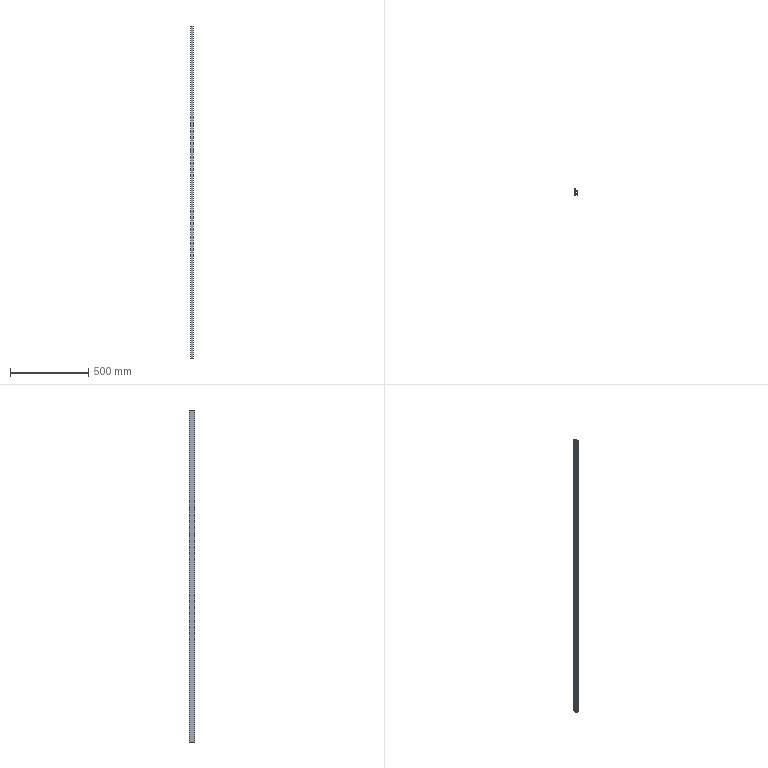Part | SolidWorks | features Extrusion 1 | 1 solid | 40 faces | box 14.605 x 34.798 x 2116 mm | volume 344207 mm3 | plane 23 | cylinder 17 | commonest cylinder face diameters 0.24 x4 0.2 x3 0.4 x2 0.5 x2 1 x2 1.2 x2
STEP:
#1=CARTESIAN_POINT('',(5.7,32.998,1058.));
#2=VERTEX_POINT('',#1);
#3=CARTESIAN_POINT('',(5.8,32.898,1058.));
#4=VERTEX_POINT('',#3);
#5=CARTESIAN_POINT('',(5.8,32.998,1058.));
#6=DIRECTION('',(0.,0.,1.));
#7=DIRECTION('',(1.,0.,0.));
#8=AXIS2_PLACEMENT_3D('',#5,#6,#7);
#9=CIRCLE('',#8,0.1);
#10=EDGE_CURVE('',#2,#4,#9,.T.);
#11=ORIENTED_EDGE('',*,*,#10,.F.);
#12=CARTESIAN_POINT('',(5.7,32.998,-1058.));
#13=VERTEX_POINT('',#12);
#14=CARTESIAN_POINT('',(5.7,32.998,1058.));
#15=DIRECTION('',(0.,0.,-1.));
#16=VECTOR('',#15,1000.);
#17=LINE('',#14,#16);
#18=EDGE_CURVE('',#2,#13,#17,.T.);
#19=ORIENTED_EDGE('',*,*,#18,.T.);
#20=CARTESIAN_POINT('',(5.8,32.898,-1058.));
#21=VERTEX_POINT('',#20);
#22=CARTESIAN_POINT('',(5.8,32.998,-1058.));
#23=DIRECTION('',(0.,0.,1.));
#24=DIRECTION('',(1.,0.,0.));
#25=AXIS2_PLACEMENT_3D('',#22,#23,#24);
#26=CIRCLE('',#25,0.1);
#27=EDGE_CURVE('',#13,#21,#26,.T.);
#28=ORIENTED_EDGE('',*,*,#27,.T.);
#29=CARTESIAN_POINT('',(5.8,32.898,1058.));
#30=DIRECTION('',(0.,0.,-1.));
#31=VECTOR('',#30,1000.);
#32=LINE('',#29,#31);
#33=EDGE_CURVE('',#4,#21,#32,.T.);
#34=ORIENTED_EDGE('',*,*,#33,.F.);
#35=EDGE_LOOP('',(#11,#19,#28,#34));
#36=FACE_OUTER_BOUND('',#35,.T.);
#37=CARTESIAN_POINT('',(5.8,32.998,1058.));
#38=DIRECTION('',(0.,0.,-1.));
#39=DIRECTION('',(-1.,0.,0.));
#40=AXIS2_PLACEMENT_3D('',#37,#38,#39);
#41=CYLINDRICAL_SURFACE('',#40,0.1);
#42=ADVANCED_FACE('',(#36),#41,.T.);
#43=CARTESIAN_POINT('',(1.75,10.,1058.));
#44=VERTEX_POINT('',#43);
#45=CARTESIAN_POINT('',(2.,10.25,1058.));
#46=VERTEX_POINT('',#45);
#47=CARTESIAN_POINT('',(2.,10.,1058.));
#48=DIRECTION('',(0.,0.,-1.));
#49=DIRECTION('',(1.,0.,0.));
#50=AXIS2_PLACEMENT_3D('',#47,#48,#49);
#51=CIRCLE('',#50,0.25);
#52=EDGE_CURVE('',#44,#46,#51,.T.);
#53=ORIENTED_EDGE('',*,*,#52,.F.);
#54=CARTESIAN_POINT('',(1.75,10.,-1058.));
#55=VERTEX_POINT('',#54);
#56=CARTESIAN_POINT('',(1.75,10.,1058.));
#57=DIRECTION('',(0.,0.,-1.));
#58=VECTOR('',#57,1000.);
#59=LINE('',#56,#58);
#60=EDGE_CURVE('',#44,#55,#59,.T.);
#61=ORIENTED_EDGE('',*,*,#60,.T.);
#62=CARTESIAN_POINT('',(2.,10.25,-1058.));
#63=VERTEX_POINT('',#62);
#64=CARTESIAN_POINT('',(2.,10.,-1058.));
#65=DIRECTION('',(0.,0.,-1.));
#66=DIRECTION('',(1.,0.,0.));
#67=AXIS2_PLACEMENT_3D('',#64,#65,#66);
#68=CIRCLE('',#67,0.25);
#69=EDGE_CURVE('',#55,#63,#68,.T.);
#70=ORIENTED_EDGE('',*,*,#69,.T.);
#71=CARTESIAN_POINT('',(2.,10.25,1058.));
#72=DIRECTION('',(0.,0.,-1.));
#73=VECTOR('',#72,1000.);
#74=LINE('',#71,#73);
#75=EDGE_CURVE('',#46,#63,#74,.T.);
#76=ORIENTED_EDGE('',*,*,#75,.F.);
#77=EDGE_LOOP('',(#53,#61,#70,#76));
#78=FACE_OUTER_BOUND('',#77,.T.);
#79=CARTESIAN_POINT('',(2.,10.,1058.));
#80=DIRECTION('',(0.,0.,-1.));
#81=DIRECTION('',(-1.,0.,0.));
#82=AXIS2_PLACEMENT_3D('',#79,#80,#81);
#83=CYLINDRICAL_SURFACE('',#82,0.25);
#84=ADVANCED_FACE('',(#78),#83,.F.);
#85=CARTESIAN_POINT('',(14.605,7.029,-1058.));
#86=VERTEX_POINT('',#85);
#87=CARTESIAN_POINT('',(14.485,7.149,-1058.));
#88=VERTEX_POINT('',#87);
#89=CARTESIAN_POINT('',(14.485,7.029,-1058.));
#90=DIRECTION('',(0.,0.,1.));
#91=DIRECTION('',(1.,0.,0.));
#92=AXIS2_PLACEMENT_3D('',#89,#90,#91);
#93=CIRCLE('',#92,0.12);
#94=EDGE_CURVE('',#86,#88,#93,.T.);
#95=ORIENTED_EDGE('',*,*,#94,.T.);
#96=CARTESIAN_POINT('',(14.485,7.149,1058.));
#97=VERTEX_POINT('',#96);
#98=CARTESIAN_POINT('',(14.485,7.149,1058.));
#99=DIRECTION('',(0.,0.,-1.));
#100=VECTOR('',#99,1000.);
#101=LINE('',#98,#100);
#102=EDGE_CURVE('',#97,#88,#101,.T.);
#103=ORIENTED_EDGE('',*,*,#102,.F.);
#104=CARTESIAN_POINT('',(14.605,7.029,1058.));
#105=VERTEX_POINT('',#104);
#106=CARTESIAN_POINT('',(14.485,7.029,1058.));
#107=DIRECTION('',(0.,0.,1.));
#108=DIRECTION('',(1.,0.,0.));
#109=AXIS2_PLACEMENT_3D('',#106,#107,#108);
#110=CIRCLE('',#109,0.12);
#111=EDGE_CURVE('',#105,#97,#110,.T.);
#112=ORIENTED_EDGE('',*,*,#111,.F.);
#113=CARTESIAN_POINT('',(14.605,7.029,1058.));
#114=DIRECTION('',(0.,0.,-1.));
#115=VECTOR('',#114,1000.);
#116=LINE('',#113,#115);
#117=EDGE_CURVE('',#105,#86,#116,.T.);
#118=ORIENTED_EDGE('',*,*,#117,.T.);
#119=EDGE_LOOP('',(#95,#103,#112,#118));
#120=FACE_OUTER_BOUND('',#119,.T.);
#121=CARTESIAN_POINT('',(14.485,7.029,1058.));
#122=DIRECTION('',(0.,0.,-1.));
#123=DIRECTION('',(-1.,0.,0.));
#124=AXIS2_PLACEMENT_3D('',#121,#122,#123);
#125=CYLINDRICAL_SURFACE('',#124,0.12);
#126=ADVANCED_FACE('',(#120),#125,.T.);
#127=CARTESIAN_POINT('',(13.705,7.149,-1058.));
#128=VERTEX_POINT('',#127);
#129=CARTESIAN_POINT('',(14.485,7.149,-1058.));
#130=DIRECTION('',(-1.,0.,0.));
#131=VECTOR('',#130,1000.);
#132=LINE('',#129,#131);
#133=EDGE_CURVE('',#88,#128,#132,.T.);
#134=ORIENTED_EDGE('',*,*,#133,.T.);
#135=CARTESIAN_POINT('',(13.705,7.149,1058.));
#136=VERTEX_POINT('',#135);
#137=CARTESIAN_POINT('',(13.705,7.149,1058.));
#138=DIRECTION('',(0.,0.,-1.));
#139=VECTOR('',#138,1000.);
#140=LINE('',#137,#139);
#141=EDGE_CURVE('',#136,#128,#140,.T.);
#142=ORIENTED_EDGE('',*,*,#141,.F.);
#143=CARTESIAN_POINT('',(14.485,7.149,1058.));
#144=DIRECTION('',(-1.,0.,0.));
#145=VECTOR('',#144,1000.);
#146=LINE('',#143,#145);
#147=EDGE_CURVE('',#97,#136,#146,.T.);
#148=ORIENTED_EDGE('',*,*,#147,.F.);
#149=ORIENTED_EDGE('',*,*,#102,.T.);
#150=EDGE_LOOP('',(#134,#142,#148,#149));
#151=FACE_OUTER_BOUND('',#150,.T.);
#152=CARTESIAN_POINT('',(14.485,7.149,1058.));
#153=DIRECTION('',(0.,-1.,0.));
#154=DIRECTION('',(0.,0.,-1.));
#155=AXIS2_PLACEMENT_3D('',#152,#153,#154);
#156=PLANE('',#155);
#157=ADVANCED_FACE('',(#151),#156,.F.);
#158=CARTESIAN_POINT('',(13.105,6.549,-1058.));
#159=VERTEX_POINT('',#158);
#160=CARTESIAN_POINT('',(13.705,6.549,-1058.));
#161=DIRECTION('',(0.,0.,1.));
#162=DIRECTION('',(1.,0.,0.));
#163=AXIS2_PLACEMENT_3D('',#160,#161,#162);
#164=CIRCLE('',#163,0.6);
#165=EDGE_CURVE('',#128,#159,#164,.T.);
#166=ORIENTED_EDGE('',*,*,#165,.T.);
#167=CARTESIAN_POINT('',(13.105,6.549,1058.));
#168=VERTEX_POINT('',#167);
#169=CARTESIAN_POINT('',(13.105,6.549,1058.));
#170=DIRECTION('',(0.,0.,-1.));
#171=VECTOR('',#170,1000.);
#172=LINE('',#169,#171);
#173=EDGE_CURVE('',#168,#159,#172,.T.);
#174=ORIENTED_EDGE('',*,*,#173,.F.);
#175=CARTESIAN_POINT('',(13.705,6.549,1058.));
#176=DIRECTION('',(0.,0.,1.));
#177=DIRECTION('',(1.,0.,0.));
#178=AXIS2_PLACEMENT_3D('',#175,#176,#177);
#179=CIRCLE('',#178,0.6);
#180=EDGE_CURVE('',#136,#168,#179,.T.);
#181=ORIENTED_EDGE('',*,*,#180,.F.);
#182=ORIENTED_EDGE('',*,*,#141,.T.);
#183=EDGE_LOOP('',(#166,#174,#181,#182));
#184=FACE_OUTER_BOUND('',#183,.T.);
#185=CARTESIAN_POINT('',(13.705,6.549,1058.));
#186=DIRECTION('',(0.,0.,-1.));
#187=DIRECTION('',(-1.,0.,0.));
#188=AXIS2_PLACEMENT_3D('',#185,#186,#187);
#189=CYLINDRICAL_SURFACE('',#188,0.6);
#190=ADVANCED_FACE('',(#184),#189,.T.);
#191=CARTESIAN_POINT('',(13.105,2.27,-1058.));
#192=VERTEX_POINT('',#191);
#193=CARTESIAN_POINT('',(13.105,6.549,-1058.));
#194=DIRECTION('',(0.,-1.,0.));
#195=VECTOR('',#194,1000.);
#196=LINE('',#193,#195);
#197=EDGE_CURVE('',#159,#192,#196,.T.);
#198=ORIENTED_EDGE('',*,*,#197,.T.);
#199=CARTESIAN_POINT('',(13.105,2.27,1058.));
#200=VERTEX_POINT('',#199);
#201=CARTESIAN_POINT('',(13.105,2.27,1058.));
#202=DIRECTION('',(0.,0.,-1.));
#203=VECTOR('',#202,1000.);
#204=LINE('',#201,#203);
#205=EDGE_CURVE('',#200,#192,#204,.T.);
#206=ORIENTED_EDGE('',*,*,#205,.F.);
#207=CARTESIAN_POINT('',(13.105,6.549,1058.));
#208=DIRECTION('',(0.,-1.,0.));
#209=VECTOR('',#208,1000.);
#210=LINE('',#207,#209);
#211=EDGE_CURVE('',#168,#200,#210,.T.);
#212=ORIENTED_EDGE('',*,*,#211,.F.);
#213=ORIENTED_EDGE('',*,*,#173,.T.);
#214=EDGE_LOOP('',(#198,#206,#212,#213));
#215=FACE_OUTER_BOUND('',#214,.T.);
#216=CARTESIAN_POINT('',(13.105,6.549,1058.));
#217=DIRECTION('',(1.,0.,0.));
#218=DIRECTION('',(0.,0.,-1.));
#219=AXIS2_PLACEMENT_3D('',#216,#217,#218);
#220=PLANE('',#219);
#221=ADVANCED_FACE('',(#215),#220,.F.);
#222=CARTESIAN_POINT('',(12.985,2.15,-1058.));
#223=VERTEX_POINT('',#222);
#224=CARTESIAN_POINT('',(12.985,2.27,-1058.));
#225=DIRECTION('',(0.,0.,-1.));
#226=DIRECTION('',(1.,0.,0.));
#227=AXIS2_PLACEMENT_3D('',#224,#225,#226);
#228=CIRCLE('',#227,0.12);
#229=EDGE_CURVE('',#192,#223,#228,.T.);
#230=ORIENTED_EDGE('',*,*,#229,.T.);
#231=CARTESIAN_POINT('',(12.985,2.15,1058.));
#232=VERTEX_POINT('',#231);
#233=CARTESIAN_POINT('',(12.985,2.15,1058.));
#234=DIRECTION('',(0.,0.,-1.));
#235=VECTOR('',#234,1000.);
#236=LINE('',#233,#235);
#237=EDGE_CURVE('',#232,#223,#236,.T.);
#238=ORIENTED_EDGE('',*,*,#237,.F.);
#239=CARTESIAN_POINT('',(12.985,2.27,1058.));
#240=DIRECTION('',(0.,0.,-1.));
#241=DIRECTION('',(1.,0.,0.));
#242=AXIS2_PLACEMENT_3D('',#239,#240,#241);
#243=CIRCLE('',#242,0.12);
#244=EDGE_CURVE('',#200,#232,#243,.T.);
#245=ORIENTED_EDGE('',*,*,#244,.F.);
#246=ORIENTED_EDGE('',*,*,#205,.T.);
#247=EDGE_LOOP('',(#230,#238,#245,#246));
#248=FACE_OUTER_BOUND('',#247,.T.);
#249=CARTESIAN_POINT('',(12.985,2.27,1058.));
#250=DIRECTION('',(0.,0.,-1.));
#251=DIRECTION('',(-1.,0.,0.));
#252=AXIS2_PLACEMENT_3D('',#249,#250,#251);
#253=CYLINDRICAL_SURFACE('',#252,0.12);
#254=ADVANCED_FACE('',(#248),#253,.F.);
#255=CARTESIAN_POINT('',(2.5,2.15,-1058.));
#256=VERTEX_POINT('',#255);
#257=CARTESIAN_POINT('',(12.985,2.15,-1058.));
#258=DIRECTION('',(-1.,0.00001466,0.));
#259=VECTOR('',#258,1000.);
#260=LINE('',#257,#259);
#261=EDGE_CURVE('',#223,#256,#260,.T.);
#262=ORIENTED_EDGE('',*,*,#261,.T.);
#263=CARTESIAN_POINT('',(2.5,2.15,1058.));
#264=VERTEX_POINT('',#263);
#265=CARTESIAN_POINT('',(2.5,2.15,1058.));
#266=DIRECTION('',(0.,0.,-1.));
#267=VECTOR('',#266,1000.);
#268=LINE('',#265,#267);
#269=EDGE_CURVE('',#264,#256,#268,.T.);
#270=ORIENTED_EDGE('',*,*,#269,.F.);
#271=CARTESIAN_POINT('',(12.985,2.15,1058.));
#272=DIRECTION('',(-1.,0.00001466,0.));
#273=VECTOR('',#272,1000.);
#274=LINE('',#271,#273);
#275=EDGE_CURVE('',#232,#264,#274,.T.);
#276=ORIENTED_EDGE('',*,*,#275,.F.);
#277=ORIENTED_EDGE('',*,*,#237,.T.);
#278=EDGE_LOOP('',(#262,#270,#276,#277));
#279=FACE_OUTER_BOUND('',#278,.T.);
#280=CARTESIAN_POINT('',(12.985,2.15,1058.));
#281=DIRECTION('',(-0.00001466,-1.,0.));
#282=DIRECTION('',(1.,-0.00001466,0.));
#283=AXIS2_PLACEMENT_3D('',#280,#281,#282);
#284=PLANE('',#283);
#285=ADVANCED_FACE('',(#279),#284,.F.);
#286=CARTESIAN_POINT('',(2.,2.65,-1058.));
#287=VERTEX_POINT('',#286);
#288=CARTESIAN_POINT('',(2.5,2.65,-1058.));
#289=DIRECTION('',(0.,0.,-1.));
#290=DIRECTION('',(1.,0.,0.));
#291=AXIS2_PLACEMENT_3D('',#288,#289,#290);
#292=CIRCLE('',#291,0.5);
#293=EDGE_CURVE('',#256,#287,#292,.T.);
#294=ORIENTED_EDGE('',*,*,#293,.T.);
#295=CARTESIAN_POINT('',(2.,2.65,1058.));
#296=VERTEX_POINT('',#295);
#297=CARTESIAN_POINT('',(2.,2.65,1058.));
#298=DIRECTION('',(0.,0.,-1.));
#299=VECTOR('',#298,1000.);
#300=LINE('',#297,#299);
#301=EDGE_CURVE('',#296,#287,#300,.T.);
#302=ORIENTED_EDGE('',*,*,#301,.F.);
#303=CARTESIAN_POINT('',(2.5,2.65,1058.));
#304=DIRECTION('',(0.,0.,-1.));
#305=DIRECTION('',(1.,0.,0.));
#306=AXIS2_PLACEMENT_3D('',#303,#304,#305);
#307=CIRCLE('',#306,0.5);
#308=EDGE_CURVE('',#264,#296,#307,.T.);
#309=ORIENTED_EDGE('',*,*,#308,.F.);
#310=ORIENTED_EDGE('',*,*,#269,.T.);
#311=EDGE_LOOP('',(#294,#302,#309,#310));
#312=FACE_OUTER_BOUND('',#311,.T.);
#313=CARTESIAN_POINT('',(2.5,2.65,1058.));
#314=DIRECTION('',(0.,0.,-1.));
#315=DIRECTION('',(-1.,0.,0.));
#316=AXIS2_PLACEMENT_3D('',#313,#314,#315);
#317=CYLINDRICAL_SURFACE('',#316,0.5);
#318=ADVANCED_FACE('',(#312),#317,.F.);
#319=CARTESIAN_POINT('',(2.,9.75,-1058.));
#320=VERTEX_POINT('',#319);
#321=CARTESIAN_POINT('',(2.,2.65,-1058.));
#322=DIRECTION('',(0.,1.,0.));
#323=VECTOR('',#322,1000.);
#324=LINE('',#321,#323);
#325=EDGE_CURVE('',#287,#320,#324,.T.);
#326=ORIENTED_EDGE('',*,*,#325,.T.);
#327=CARTESIAN_POINT('',(2.,9.75,1058.));
#328=VERTEX_POINT('',#327);
#329=CARTESIAN_POINT('',(2.,9.75,1058.));
#330=DIRECTION('',(0.,0.,-1.));
#331=VECTOR('',#330,1000.);
#332=LINE('',#329,#331);
#333=EDGE_CURVE('',#328,#320,#332,.T.);
#334=ORIENTED_EDGE('',*,*,#333,.F.);
#335=CARTESIAN_POINT('',(2.,2.65,1058.));
#336=DIRECTION('',(0.,1.,0.));
#337=VECTOR('',#336,1000.);
#338=LINE('',#335,#337);
#339=EDGE_CURVE('',#296,#328,#338,.T.);
#340=ORIENTED_EDGE('',*,*,#339,.F.);
#341=ORIENTED_EDGE('',*,*,#301,.T.);
#342=EDGE_LOOP('',(#326,#334,#340,#341));
#343=FACE_OUTER_BOUND('',#342,.T.);
#344=CARTESIAN_POINT('',(2.,2.65,1058.));
#345=DIRECTION('',(-1.,0.,0.));
#346=DIRECTION('',(0.,0.,1.));
#347=AXIS2_PLACEMENT_3D('',#344,#345,#346);
#348=PLANE('',#347);
#349=ADVANCED_FACE('',(#343),#348,.F.);
#350=ORIENTED_EDGE('',*,*,#60,.F.);
#351=CARTESIAN_POINT('',(2.,10.,1058.));
#352=DIRECTION('',(0.,0.,-1.));
#353=DIRECTION('',(1.,0.,0.));
#354=AXIS2_PLACEMENT_3D('',#351,#352,#353);
#355=CIRCLE('',#354,0.25);
#356=EDGE_CURVE('',#328,#44,#355,.T.);
#357=ORIENTED_EDGE('',*,*,#356,.F.);
#358=ORIENTED_EDGE('',*,*,#333,.T.);
#359=CARTESIAN_POINT('',(2.,10.,-1058.));
#360=DIRECTION('',(0.,0.,-1.));
#361=DIRECTION('',(1.,0.,0.));
#362=AXIS2_PLACEMENT_3D('',#359,#360,#361);
#363=CIRCLE('',#362,0.25);
#364=EDGE_CURVE('',#320,#55,#363,.T.);
#365=ORIENTED_EDGE('',*,*,#364,.T.);
#366=EDGE_LOOP('',(#350,#357,#358,#365));
#367=FACE_OUTER_BOUND('',#366,.T.);
#368=CARTESIAN_POINT('',(2.,10.,1058.));
#369=DIRECTION('',(0.,0.,-1.));
#370=DIRECTION('',(-1.,0.,0.));
#371=AXIS2_PLACEMENT_3D('',#368,#369,#370);
#372=CYLINDRICAL_SURFACE('',#371,0.25);
#373=ADVANCED_FACE('',(#367),#372,.F.);
#374=CARTESIAN_POINT('',(2.,17.35,-1058.));
#375=VERTEX_POINT('',#374);
#376=CARTESIAN_POINT('',(2.,10.25,-1058.));
#377=DIRECTION('',(0.,1.,0.));
#378=VECTOR('',#377,1000.);
#379=LINE('',#376,#378);
#380=EDGE_CURVE('',#63,#375,#379,.T.);
#381=ORIENTED_EDGE('',*,*,#380,.T.);
#382=CARTESIAN_POINT('',(2.,17.35,1058.));
#383=VERTEX_POINT('',#382);
#384=CARTESIAN_POINT('',(2.,17.35,1058.));
#385=DIRECTION('',(0.,0.,-1.));
#386=VECTOR('',#385,1000.);
#387=LINE('',#384,#386);
#388=EDGE_CURVE('',#383,#375,#387,.T.);
#389=ORIENTED_EDGE('',*,*,#388,.F.);
#390=CARTESIAN_POINT('',(2.,10.25,1058.));
#391=DIRECTION('',(0.,1.,0.));
#392=VECTOR('',#391,1000.);
#393=LINE('',#390,#392);
#394=EDGE_CURVE('',#46,#383,#393,.T.);
#395=ORIENTED_EDGE('',*,*,#394,.F.);
#396=ORIENTED_EDGE('',*,*,#75,.T.);
#397=EDGE_LOOP('',(#381,#389,#395,#396));
#398=FACE_OUTER_BOUND('',#397,.T.);
#399=CARTESIAN_POINT('',(2.,10.25,1058.));
#400=DIRECTION('',(-1.,0.,0.));
#401=DIRECTION('',(0.,0.,1.));
#402=AXIS2_PLACEMENT_3D('',#399,#400,#401);
#403=PLANE('',#402);
#404=ADVANCED_FACE('',(#398),#403,.F.);
#405=CARTESIAN_POINT('',(2.5,17.85,-1058.));
#406=VERTEX_POINT('',#405);
#407=CARTESIAN_POINT('',(2.5,17.35,-1058.));
#408=DIRECTION('',(0.,0.,-1.));
#409=DIRECTION('',(1.,0.,0.));
#410=AXIS2_PLACEMENT_3D('',#407,#408,#409);
#411=CIRCLE('',#410,0.5);
#412=EDGE_CURVE('',#375,#406,#411,.T.);
#413=ORIENTED_EDGE('',*,*,#412,.T.);
#414=CARTESIAN_POINT('',(2.5,17.85,1058.));
#415=VERTEX_POINT('',#414);
#416=CARTESIAN_POINT('',(2.5,17.85,1058.));
#417=DIRECTION('',(0.,0.,-1.));
#418=VECTOR('',#417,1000.);
#419=LINE('',#416,#418);
#420=EDGE_CURVE('',#415,#406,#419,.T.);
#421=ORIENTED_EDGE('',*,*,#420,.F.);
#422=CARTESIAN_POINT('',(2.5,17.35,1058.));
#423=DIRECTION('',(0.,0.,-1.));
#424=DIRECTION('',(1.,0.,0.));
#425=AXIS2_PLACEMENT_3D('',#422,#423,#424);
#426=CIRCLE('',#425,0.5);
#427=EDGE_CURVE('',#383,#415,#426,.T.);
#428=ORIENTED_EDGE('',*,*,#427,.F.);
#429=ORIENTED_EDGE('',*,*,#388,.T.);
#430=EDGE_LOOP('',(#413,#421,#428,#429));
#431=FACE_OUTER_BOUND('',#430,.T.);
#432=CARTESIAN_POINT('',(2.5,17.35,1058.));
#433=DIRECTION('',(0.,0.,-1.));
#434=DIRECTION('',(-1.,0.,0.));
#435=AXIS2_PLACEMENT_3D('',#432,#433,#434);
#436=CYLINDRICAL_SURFACE('',#435,0.5);
#437=ADVANCED_FACE('',(#431),#436,.F.);
#438=CARTESIAN_POINT('',(14.604,17.85,-1058.));
#439=VERTEX_POINT('',#438);
#440=CARTESIAN_POINT('',(2.5,17.85,-1058.));
#441=DIRECTION('',(1.,0.,0.));
#442=VECTOR('',#441,1000.);
#443=LINE('',#440,#442);
#444=EDGE_CURVE('',#406,#439,#443,.T.);
#445=ORIENTED_EDGE('',*,*,#444,.T.);
#446=CARTESIAN_POINT('',(14.604,17.85,1058.));
#447=VERTEX_POINT('',#446);
#448=CARTESIAN_POINT('',(14.604,17.85,1058.));
#449=DIRECTION('',(0.,0.,-1.));
#450=VECTOR('',#449,1000.);
#451=LINE('',#448,#450);
#452=EDGE_CURVE('',#447,#439,#451,.T.);
#453=ORIENTED_EDGE('',*,*,#452,.F.);
#454=CARTESIAN_POINT('',(2.5,17.85,1058.));
#455=DIRECTION('',(1.,0.,0.));
#456=VECTOR('',#455,1000.);
#457=LINE('',#454,#456);
#458=EDGE_CURVE('',#415,#447,#457,.T.);
#459=ORIENTED_EDGE('',*,*,#458,.F.);
#460=ORIENTED_EDGE('',*,*,#420,.T.);
#461=EDGE_LOOP('',(#445,#453,#459,#460));
#462=FACE_OUTER_BOUND('',#461,.T.);
#463=CARTESIAN_POINT('',(2.5,17.85,1058.));
#464=DIRECTION('',(0.,1.,0.));
#465=DIRECTION('',(0.,0.,1.));
#466=AXIS2_PLACEMENT_3D('',#463,#464,#465);
#467=PLANE('',#466);
#468=ADVANCED_FACE('',(#462),#467,.F.);
#469=CARTESIAN_POINT('',(14.604,23.83,-1058.));
#470=VERTEX_POINT('',#469);
#471=CARTESIAN_POINT('',(14.604,17.85,-1058.));
#472=DIRECTION('',(0.,1.,0.));
#473=VECTOR('',#472,1000.);
#474=LINE('',#471,#473);
#475=EDGE_CURVE('',#439,#470,#474,.T.);
#476=ORIENTED_EDGE('',*,*,#475,.T.);
#477=CARTESIAN_POINT('',(14.604,23.83,1058.));
#478=VERTEX_POINT('',#477);
#479=CARTESIAN_POINT('',(14.604,23.83,1058.));
#480=DIRECTION('',(0.,0.,-1.));
#481=VECTOR('',#480,1000.);
#482=LINE('',#479,#481);
#483=EDGE_CURVE('',#478,#470,#482,.T.);
#484=ORIENTED_EDGE('',*,*,#483,.F.);
#485=CARTESIAN_POINT('',(14.604,17.85,1058.));
#486=DIRECTION('',(0.,1.,0.));
#487=VECTOR('',#486,1000.);
#488=LINE('',#485,#487);
#489=EDGE_CURVE('',#447,#478,#488,.T.);
#490=ORIENTED_EDGE('',*,*,#489,.F.);
#491=ORIENTED_EDGE('',*,*,#452,.T.);
#492=EDGE_LOOP('',(#476,#484,#490,#491));
#493=FACE_OUTER_BOUND('',#492,.T.);
#494=CARTESIAN_POINT('',(14.604,17.85,1058.));
#495=DIRECTION('',(-1.,0.,0.));
#496=DIRECTION('',(0.,0.,1.));
#497=AXIS2_PLACEMENT_3D('',#494,#495,#496);
#498=PLANE('',#497);
#499=ADVANCED_FACE('',(#493),#498,.F.);
#500=CARTESIAN_POINT('',(14.484,23.95,-1058.));
#501=VERTEX_POINT('',#500);
#502=CARTESIAN_POINT('',(14.484,23.83,-1058.));
#503=DIRECTION('',(0.,0.,1.));
#504=DIRECTION('',(1.,0.,0.));
#505=AXIS2_PLACEMENT_3D('',#502,#503,#504);
#506=CIRCLE('',#505,0.12);
#507=EDGE_CURVE('',#470,#501,#506,.T.);
#508=ORIENTED_EDGE('',*,*,#507,.T.);
#509=CARTESIAN_POINT('',(14.484,23.95,1058.));
#510=VERTEX_POINT('',#509);
#511=CARTESIAN_POINT('',(14.484,23.95,1058.));
#512=DIRECTION('',(0.,0.,-1.));
#513=VECTOR('',#512,1000.);
#514=LINE('',#511,#513);
#515=EDGE_CURVE('',#510,#501,#514,.T.);
#516=ORIENTED_EDGE('',*,*,#515,.F.);
#517=CARTESIAN_POINT('',(14.484,23.83,1058.));
#518=DIRECTION('',(0.,0.,1.));
#519=DIRECTION('',(1.,0.,0.));
#520=AXIS2_PLACEMENT_3D('',#517,#518,#519);
#521=CIRCLE('',#520,0.12);
#522=EDGE_CURVE('',#478,#510,#521,.T.);
#523=ORIENTED_EDGE('',*,*,#522,.F.);
#524=ORIENTED_EDGE('',*,*,#483,.T.);
#525=EDGE_LOOP('',(#508,#516,#523,#524));
#526=FACE_OUTER_BOUND('',#525,.T.);
#527=CARTESIAN_POINT('',(14.484,23.83,1058.));
#528=DIRECTION('',(0.,0.,-1.));
#529=DIRECTION('',(-1.,0.,0.));
#530=AXIS2_PLACEMENT_3D('',#527,#528,#529);
#531=CYLINDRICAL_SURFACE('',#530,0.12);
#532=ADVANCED_FACE('',(#526),#531,.T.);
#533=CARTESIAN_POINT('',(13.704,23.95,-1058.));
#534=VERTEX_POINT('',#533);
#535=CARTESIAN_POINT('',(14.484,23.95,-1058.));
#536=DIRECTION('',(-1.,0.,0.));
#537=VECTOR('',#536,1000.);
#538=LINE('',#535,#537);
#539=EDGE_CURVE('',#501,#534,#538,.T.);
#540=ORIENTED_EDGE('',*,*,#539,.T.);
#541=CARTESIAN_POINT('',(13.704,23.95,1058.));
#542=VERTEX_POINT('',#541);
#543=CARTESIAN_POINT('',(13.704,23.95,1058.));
#544=DIRECTION('',(0.,0.,-1.));
#545=VECTOR('',#544,1000.);
#546=LINE('',#543,#545);
#547=EDGE_CURVE('',#542,#534,#546,.T.);
#548=ORIENTED_EDGE('',*,*,#547,.F.);
#549=CARTESIAN_POINT('',(14.484,23.95,1058.));
#550=DIRECTION('',(-1.,0.,0.));
#551=VECTOR('',#550,1000.);
#552=LINE('',#549,#551);
#553=EDGE_CURVE('',#510,#542,#552,.T.);
#554=ORIENTED_EDGE('',*,*,#553,.F.);
#555=ORIENTED_EDGE('',*,*,#515,.T.);
#556=EDGE_LOOP('',(#540,#548,#554,#555));
#557=FACE_OUTER_BOUND('',#556,.T.);
#558=CARTESIAN_POINT('',(14.484,23.95,1058.));
#559=DIRECTION('',(0.,-1.,0.));
#560=DIRECTION('',(0.,0.,-1.));
#561=AXIS2_PLACEMENT_3D('',#558,#559,#560);
#562=PLANE('',#561);
#563=ADVANCED_FACE('',(#557),#562,.F.);
#564=CARTESIAN_POINT('',(13.104,23.35,-1058.));
#565=VERTEX_POINT('',#564);
#566=CARTESIAN_POINT('',(13.704,23.35,-1058.));
#567=DIRECTION('',(0.,0.,1.));
#568=DIRECTION('',(1.,0.,0.));
#569=AXIS2_PLACEMENT_3D('',#566,#567,#568);
#570=CIRCLE('',#569,0.6);
#571=EDGE_CURVE('',#534,#565,#570,.T.);
#572=ORIENTED_EDGE('',*,*,#571,.T.);
#573=CARTESIAN_POINT('',(13.104,23.35,1058.));
#574=VERTEX_POINT('',#573);
#575=CARTESIAN_POINT('',(13.104,23.35,1058.));
#576=DIRECTION('',(0.,0.,-1.));
#577=VECTOR('',#576,1000.);
#578=LINE('',#575,#577);
#579=EDGE_CURVE('',#574,#565,#578,.T.);
#580=ORIENTED_EDGE('',*,*,#579,.F.);
#581=CARTESIAN_POINT('',(13.704,23.35,1058.));
#582=DIRECTION('',(0.,0.,1.));
#583=DIRECTION('',(1.,0.,0.));
#584=AXIS2_PLACEMENT_3D('',#581,#582,#583);
#585=CIRCLE('',#584,0.6);
#586=EDGE_CURVE('',#542,#574,#585,.T.);
#587=ORIENTED_EDGE('',*,*,#586,.F.);
#588=ORIENTED_EDGE('',*,*,#547,.T.);
#589=EDGE_LOOP('',(#572,#580,#587,#588));
#590=FACE_OUTER_BOUND('',#589,.T.);
#591=CARTESIAN_POINT('',(13.704,23.35,1058.));
#592=DIRECTION('',(0.,0.,-1.));
#593=DIRECTION('',(-1.,0.,0.));
#594=AXIS2_PLACEMENT_3D('',#591,#592,#593);
#595=CYLINDRICAL_SURFACE('',#594,0.6);
#596=ADVANCED_FACE('',(#590),#595,.T.);
#597=CARTESIAN_POINT('',(13.104,19.47,-1058.));
#598=VERTEX_POINT('',#597);
#599=CARTESIAN_POINT('',(13.104,23.35,-1058.));
#600=DIRECTION('',(0.,-1.,0.));
#601=VECTOR('',#600,1000.);
#602=LINE('',#599,#601);
#603=EDGE_CURVE('',#565,#598,#602,.T.);
#604=ORIENTED_EDGE('',*,*,#603,.T.);
#605=CARTESIAN_POINT('',(13.104,19.47,1058.));
#606=VERTEX_POINT('',#605);
#607=CARTESIAN_POINT('',(13.104,19.47,1058.));
#608=DIRECTION('',(0.,0.,-1.));
#609=VECTOR('',#608,1000.);
#610=LINE('',#607,#609);
#611=EDGE_CURVE('',#606,#598,#610,.T.);
#612=ORIENTED_EDGE('',*,*,#611,.F.);
#613=CARTESIAN_POINT('',(13.104,23.35,1058.));
#614=DIRECTION('',(0.,-1.,0.));
#615=VECTOR('',#614,1000.);
#616=LINE('',#613,#615);
#617=EDGE_CURVE('',#574,#606,#616,.T.);
#618=ORIENTED_EDGE('',*,*,#617,.F.);
#619=ORIENTED_EDGE('',*,*,#579,.T.);
#620=EDGE_LOOP('',(#604,#612,#618,#619));
#621=FACE_OUTER_BOUND('',#620,.T.);
#622=CARTESIAN_POINT('',(13.104,23.35,1058.));
#623=DIRECTION('',(1.,0.,0.));
#624=DIRECTION('',(0.,0.,-1.));
#625=AXIS2_PLACEMENT_3D('',#622,#623,#624);
#626=PLANE('',#625);
#627=ADVANCED_FACE('',(#621),#626,.F.);
#628=CARTESIAN_POINT('',(12.984,19.35,-1058.));
#629=VERTEX_POINT('',#628);
#630=CARTESIAN_POINT('',(12.984,19.47,-1058.));
#631=DIRECTION('',(0.,0.,-1.));
#632=DIRECTION('',(1.,0.,0.));
#633=AXIS2_PLACEMENT_3D('',#630,#631,#632);
#634=CIRCLE('',#633,0.12);
#635=EDGE_CURVE('',#598,#629,#634,.T.);
#636=ORIENTED_EDGE('',*,*,#635,.T.);
#637=CARTESIAN_POINT('',(12.984,19.35,1058.));
#638=VERTEX_POINT('',#637);
#639=CARTESIAN_POINT('',(12.984,19.35,1058.));
#640=DIRECTION('',(0.,0.,-1.));
#641=VECTOR('',#640,1000.);
#642=LINE('',#639,#641);
#643=EDGE_CURVE('',#638,#629,#642,.T.);
#644=ORIENTED_EDGE('',*,*,#643,.F.);
#645=CARTESIAN_POINT('',(12.984,19.47,1058.));
#646=DIRECTION('',(0.,0.,-1.));
#647=DIRECTION('',(1.,0.,0.));
#648=AXIS2_PLACEMENT_3D('',#645,#646,#647);
#649=CIRCLE('',#648,0.12);
#650=EDGE_CURVE('',#606,#638,#649,.T.);
#651=ORIENTED_EDGE('',*,*,#650,.F.);
#652=ORIENTED_EDGE('',*,*,#611,.T.);
#653=EDGE_LOOP('',(#636,#644,#651,#652));
#654=FACE_OUTER_BOUND('',#653,.T.);
#655=CARTESIAN_POINT('',(12.984,19.47,1058.));
#656=DIRECTION('',(0.,0.,-1.));
#657=DIRECTION('',(-1.,0.,0.));
#658=AXIS2_PLACEMENT_3D('',#655,#656,#657);
#659=CYLINDRICAL_SURFACE('',#658,0.12);
#660=ADVANCED_FACE('',(#654),#659,.F.);
#661=CARTESIAN_POINT('',(7.2,19.35,-1058.));
#662=VERTEX_POINT('',#661);
#663=CARTESIAN_POINT('',(12.984,19.35,-1058.));
#664=DIRECTION('',(-1.,0.,0.));
#665=VECTOR('',#664,1000.);
#666=LINE('',#663,#665);
#667=EDGE_CURVE('',#629,#662,#666,.T.);
#668=ORIENTED_EDGE('',*,*,#667,.T.);
#669=CARTESIAN_POINT('',(7.2,19.35,1058.));
#670=VERTEX_POINT('',#669);
#671=CARTESIAN_POINT('',(7.2,19.35,1058.));
#672=DIRECTION('',(0.,0.,-1.));
#673=VECTOR('',#672,1000.);
#674=LINE('',#671,#673);
#675=EDGE_CURVE('',#670,#662,#674,.T.);
#676=ORIENTED_EDGE('',*,*,#675,.F.);
#677=CARTESIAN_POINT('',(12.984,19.35,1058.));
#678=DIRECTION('',(-1.,0.,0.));
#679=VECTOR('',#678,1000.);
#680=LINE('',#677,#679);
#681=EDGE_CURVE('',#638,#670,#680,.T.);
#682=ORIENTED_EDGE('',*,*,#681,.F.);
#683=ORIENTED_EDGE('',*,*,#643,.T.);
#684=EDGE_LOOP('',(#668,#676,#682,#683));
#685=FACE_OUTER_BOUND('',#684,.T.);
#686=CARTESIAN_POINT('',(12.984,19.35,1058.));
#687=DIRECTION('',(0.,-1.,0.));
#688=DIRECTION('',(0.,0.,-1.));
#689=AXIS2_PLACEMENT_3D('',#686,#687,#688);
#690=PLANE('',#689);
#691=ADVANCED_FACE('',(#685),#690,.F.);
#692=CARTESIAN_POINT('',(7.2,34.798,-1058.));
#693=VERTEX_POINT('',#692);
#694=CARTESIAN_POINT('',(7.2,19.35,-1058.));
#695=DIRECTION('',(0.,1.,0.));
#696=VECTOR('',#695,1000.);
#697=LINE('',#694,#696);
#698=EDGE_CURVE('',#662,#693,#697,.T.);
#699=ORIENTED_EDGE('',*,*,#698,.T.);
#700=CARTESIAN_POINT('',(7.2,34.798,1058.));
#701=VERTEX_POINT('',#700);
#702=CARTESIAN_POINT('',(7.2,34.798,1058.));
#703=DIRECTION('',(0.,0.,-1.));
#704=VECTOR('',#703,1000.);
#705=LINE('',#702,#704);
#706=EDGE_CURVE('',#701,#693,#705,.T.);
#707=ORIENTED_EDGE('',*,*,#706,.F.);
#708=CARTESIAN_POINT('',(7.2,19.35,1058.));
#709=DIRECTION('',(0.,1.,0.));
#710=VECTOR('',#709,1000.);
#711=LINE('',#708,#710);
#712=EDGE_CURVE('',#670,#701,#711,.T.);
#713=ORIENTED_EDGE('',*,*,#712,.F.);
#714=ORIENTED_EDGE('',*,*,#675,.T.);
#715=EDGE_LOOP('',(#699,#707,#713,#714));
#716=FACE_OUTER_BOUND('',#715,.T.);
#717=CARTESIAN_POINT('',(7.2,19.35,1058.));
#718=DIRECTION('',(-1.,0.,0.));
#719=DIRECTION('',(0.,0.,1.));
#720=AXIS2_PLACEMENT_3D('',#717,#718,#719);
#721=PLANE('',#720);
#722=ADVANCED_FACE('',(#716),#721,.F.);
#723=CARTESIAN_POINT('',(6.,34.798,-1058.));
#724=VERTEX_POINT('',#723);
#725=CARTESIAN_POINT('',(7.2,34.798,-1058.));
#726=DIRECTION('',(-1.,0.,0.));
#727=VECTOR('',#726,1000.);
#728=LINE('',#725,#727);
#729=EDGE_CURVE('',#693,#724,#728,.T.);
#730=ORIENTED_EDGE('',*,*,#729,.T.);
#731=CARTESIAN_POINT('',(6.,34.798,1058.));
#732=VERTEX_POINT('',#731);
#733=CARTESIAN_POINT('',(6.,34.798,1058.));
#734=DIRECTION('',(0.,0.,-1.));
#735=VECTOR('',#734,1000.);
#736=LINE('',#733,#735);
#737=EDGE_CURVE('',#732,#724,#736,.T.);
#738=ORIENTED_EDGE('',*,*,#737,.F.);
#739=CARTESIAN_POINT('',(7.2,34.798,1058.));
#740=DIRECTION('',(-1.,0.,0.));
#741=VECTOR('',#740,1000.);
#742=LINE('',#739,#741);
#743=EDGE_CURVE('',#701,#732,#742,.T.);
#744=ORIENTED_EDGE('',*,*,#743,.F.);
#745=ORIENTED_EDGE('',*,*,#706,.T.);
#746=EDGE_LOOP('',(#730,#738,#744,#745));
#747=FACE_OUTER_BOUND('',#746,.T.);
#748=CARTESIAN_POINT('',(7.2,34.798,1058.));
#749=DIRECTION('',(0.,-1.,0.));
#750=DIRECTION('',(0.,0.,-1.));
#751=AXIS2_PLACEMENT_3D('',#748,#749,#750);
#752=PLANE('',#751);
#753=ADVANCED_FACE('',(#747),#752,.F.);
#754=CARTESIAN_POINT('',(5.8,34.598,-1058.));
#755=VERTEX_POINT('',#754);
#756=CARTESIAN_POINT('',(6.,34.598,-1058.));
#757=DIRECTION('',(0.,0.,1.));
#758=DIRECTION('',(1.,0.,0.));
#759=AXIS2_PLACEMENT_3D('',#756,#757,#758);
#760=CIRCLE('',#759,0.2);
#761=EDGE_CURVE('',#724,#755,#760,.T.);
#762=ORIENTED_EDGE('',*,*,#761,.T.);
#763=CARTESIAN_POINT('',(5.8,34.598,1058.));
#764=VERTEX_POINT('',#763);
#765=CARTESIAN_POINT('',(5.8,34.598,1058.));
#766=DIRECTION('',(0.,0.,-1.));
#767=VECTOR('',#766,1000.);
#768=LINE('',#765,#767);
#769=EDGE_CURVE('',#764,#755,#768,.T.);
#770=ORIENTED_EDGE('',*,*,#769,.F.);
#771=CARTESIAN_POINT('',(6.,34.598,1058.));
#772=DIRECTION('',(0.,0.,1.));
#773=DIRECTION('',(1.,0.,0.));
#774=AXIS2_PLACEMENT_3D('',#771,#772,#773);
#775=CIRCLE('',#774,0.2);
#776=EDGE_CURVE('',#732,#764,#775,.T.);
#777=ORIENTED_EDGE('',*,*,#776,.F.);
#778=ORIENTED_EDGE('',*,*,#737,.T.);
#779=EDGE_LOOP('',(#762,#770,#777,#778));
#780=FACE_OUTER_BOUND('',#779,.T.);
#781=CARTESIAN_POINT('',(6.,34.598,1058.));
#782=DIRECTION('',(0.,0.,-1.));
#783=DIRECTION('',(-1.,0.,0.));
#784=AXIS2_PLACEMENT_3D('',#781,#782,#783);
#785=CYLINDRICAL_SURFACE('',#784,0.2);
#786=ADVANCED_FACE('',(#780),#785,.T.);
#787=CARTESIAN_POINT('',(5.8,33.098,-1058.));
#788=VERTEX_POINT('',#787);
#789=CARTESIAN_POINT('',(5.8,34.598,-1058.));
#790=DIRECTION('',(0.,-1.,0.));
#791=VECTOR('',#790,1000.);
#792=LINE('',#789,#791);
#793=EDGE_CURVE('',#755,#788,#792,.T.);
#794=ORIENTED_EDGE('',*,*,#793,.T.);
#795=CARTESIAN_POINT('',(5.8,33.098,1058.));
#796=VERTEX_POINT('',#795);
#797=CARTESIAN_POINT('',(5.8,33.098,1058.));
#798=DIRECTION('',(0.,0.,-1.));
#799=VECTOR('',#798,1000.);
#800=LINE('',#797,#799);
#801=EDGE_CURVE('',#796,#788,#800,.T.);
#802=ORIENTED_EDGE('',*,*,#801,.F.);
#803=CARTESIAN_POINT('',(5.8,34.598,1058.));
#804=DIRECTION('',(0.,-1.,0.));
#805=VECTOR('',#804,1000.);
#806=LINE('',#803,#805);
#807=EDGE_CURVE('',#764,#796,#806,.T.);
#808=ORIENTED_EDGE('',*,*,#807,.F.);
#809=ORIENTED_EDGE('',*,*,#769,.T.);
#810=EDGE_LOOP('',(#794,#802,#808,#809));
#811=FACE_OUTER_BOUND('',#810,.T.);
#812=CARTESIAN_POINT('',(5.8,34.598,1058.));
#813=DIRECTION('',(1.,0.,0.));
#814=DIRECTION('',(0.,0.,-1.));
#815=AXIS2_PLACEMENT_3D('',#812,#813,#814);
#816=PLANE('',#815);
#817=ADVANCED_FACE('',(#811),#816,.F.);
#818=ORIENTED_EDGE('',*,*,#18,.F.);
#819=CARTESIAN_POINT('',(5.8,32.998,1058.));
#820=DIRECTION('',(0.,0.,1.));
#821=DIRECTION('',(1.,0.,0.));
#822=AXIS2_PLACEMENT_3D('',#819,#820,#821);
#823=CIRCLE('',#822,0.1);
#824=EDGE_CURVE('',#796,#2,#823,.T.);
#825=ORIENTED_EDGE('',*,*,#824,.F.);
#826=ORIENTED_EDGE('',*,*,#801,.T.);
#827=CARTESIAN_POINT('',(5.8,32.998,-1058.));
#828=DIRECTION('',(0.,0.,1.));
#829=DIRECTION('',(1.,0.,0.));
#830=AXIS2_PLACEMENT_3D('',#827,#828,#829);
#831=CIRCLE('',#830,0.1);
#832=EDGE_CURVE('',#788,#13,#831,.T.);
#833=ORIENTED_EDGE('',*,*,#832,.T.);
#834=EDGE_LOOP('',(#818,#825,#826,#833));
#835=FACE_OUTER_BOUND('',#834,.T.);
#836=CARTESIAN_POINT('',(5.8,32.998,1058.));
#837=DIRECTION('',(0.,0.,-1.));
#838=DIRECTION('',(-1.,0.,0.));
#839=AXIS2_PLACEMENT_3D('',#836,#837,#838);
#840=CYLINDRICAL_SURFACE('',#839,0.1);
#841=ADVANCED_FACE('',(#835),#840,.T.);
#842=CARTESIAN_POINT('',(5.8,23.812,-1058.));
#843=VERTEX_POINT('',#842);
#844=CARTESIAN_POINT('',(5.8,32.898,-1058.));
#845=DIRECTION('',(0.,-1.,0.));
#846=VECTOR('',#845,1000.);
#847=LINE('',#844,#846);
#848=EDGE_CURVE('',#21,#843,#847,.T.);
#849=ORIENTED_EDGE('',*,*,#848,.T.);
#850=CARTESIAN_POINT('',(5.8,23.812,1058.));
#851=VERTEX_POINT('',#850);
#852=CARTESIAN_POINT('',(5.8,23.812,1058.));
#853=DIRECTION('',(0.,0.,-1.));
#854=VECTOR('',#853,1000.);
#855=LINE('',#852,#854);
#856=EDGE_CURVE('',#851,#843,#855,.T.);
#857=ORIENTED_EDGE('',*,*,#856,.F.);
#858=CARTESIAN_POINT('',(5.8,32.898,1058.));
#859=DIRECTION('',(0.,-1.,0.));
#860=VECTOR('',#859,1000.);
#861=LINE('',#858,#860);
#862=EDGE_CURVE('',#4,#851,#861,.T.);
#863=ORIENTED_EDGE('',*,*,#862,.F.);
#864=ORIENTED_EDGE('',*,*,#33,.T.);
#865=EDGE_LOOP('',(#849,#857,#863,#864));
#866=FACE_OUTER_BOUND('',#865,.T.);
#867=CARTESIAN_POINT('',(5.8,32.898,1058.));
#868=DIRECTION('',(1.,0.,0.));
#869=DIRECTION('',(0.,0.,-1.));
#870=AXIS2_PLACEMENT_3D('',#867,#868,#869);
#871=PLANE('',#870);
#872=ADVANCED_FACE('',(#866),#871,.F.);
#873=CARTESIAN_POINT('',(4.8,22.812,-1058.));
#874=VERTEX_POINT('',#873);
#875=CARTESIAN_POINT('',(4.8,23.812,-1058.));
#876=DIRECTION('',(0.,0.,-1.));
#877=DIRECTION('',(1.,0.,0.));
#878=AXIS2_PLACEMENT_3D('',#875,#876,#877);
#879=CIRCLE('',#878,1.);
#880=EDGE_CURVE('',#843,#874,#879,.T.);
#881=ORIENTED_EDGE('',*,*,#880,.T.);
#882=CARTESIAN_POINT('',(4.8,22.812,1058.));
#883=VERTEX_POINT('',#882);
#884=CARTESIAN_POINT('',(4.8,22.812,1058.));
#885=DIRECTION('',(0.,0.,-1.));
#886=VECTOR('',#885,1000.);
#887=LINE('',#884,#886);
#888=EDGE_CURVE('',#883,#874,#887,.T.);
#889=ORIENTED_EDGE('',*,*,#888,.F.);
#890=CARTESIAN_POINT('',(4.8,23.812,1058.));
#891=DIRECTION('',(0.,0.,-1.));
#892=DIRECTION('',(1.,0.,0.));
#893=AXIS2_PLACEMENT_3D('',#890,#891,#892);
#894=CIRCLE('',#893,1.);
#895=EDGE_CURVE('',#851,#883,#894,.T.);
#896=ORIENTED_EDGE('',*,*,#895,.F.);
#897=ORIENTED_EDGE('',*,*,#856,.T.);
#898=EDGE_LOOP('',(#881,#889,#896,#897));
#899=FACE_OUTER_BOUND('',#898,.T.);
#900=CARTESIAN_POINT('',(4.8,23.812,1058.));
#901=DIRECTION('',(0.,0.,-1.));
#902=DIRECTION('',(-1.,0.,0.));
#903=AXIS2_PLACEMENT_3D('',#900,#901,#902);
#904=CYLINDRICAL_SURFACE('',#903,1.);
#905=ADVANCED_FACE('',(#899),#904,.F.);
#906=CARTESIAN_POINT('',(2.8,22.812,-1058.));
#907=VERTEX_POINT('',#906);
#908=CARTESIAN_POINT('',(4.8,22.812,-1058.));
#909=DIRECTION('',(-1.,0.,0.));
#910=VECTOR('',#909,1000.);
#911=LINE('',#908,#910);
#912=EDGE_CURVE('',#874,#907,#911,.T.);
#913=ORIENTED_EDGE('',*,*,#912,.T.);
#914=CARTESIAN_POINT('',(2.8,22.812,1058.));
#915=VERTEX_POINT('',#914);
#916=CARTESIAN_POINT('',(2.8,22.812,1058.));
#917=DIRECTION('',(0.,0.,-1.));
#918=VECTOR('',#917,1000.);
#919=LINE('',#916,#918);
#920=EDGE_CURVE('',#915,#907,#919,.T.);
#921=ORIENTED_EDGE('',*,*,#920,.F.);
#922=CARTESIAN_POINT('',(4.8,22.812,1058.));
#923=DIRECTION('',(-1.,0.,0.));
#924=VECTOR('',#923,1000.);
#925=LINE('',#922,#924);
#926=EDGE_CURVE('',#883,#915,#925,.T.);
#927=ORIENTED_EDGE('',*,*,#926,.F.);
#928=ORIENTED_EDGE('',*,*,#888,.T.);
#929=EDGE_LOOP('',(#913,#921,#927,#928));
#930=FACE_OUTER_BOUND('',#929,.T.);
#931=CARTESIAN_POINT('',(4.8,22.812,1058.));
#932=DIRECTION('',(0.,-1.,0.));
#933=DIRECTION('',(0.,0.,-1.));
#934=AXIS2_PLACEMENT_3D('',#931,#932,#933);
#935=PLANE('',#934);
#936=ADVANCED_FACE('',(#930),#935,.F.);
#937=CARTESIAN_POINT('',(1.8,23.812,-1058.));
#938=VERTEX_POINT('',#937);
#939=CARTESIAN_POINT('',(2.8,23.812,-1058.));
#940=DIRECTION('',(0.,0.,-1.));
#941=DIRECTION('',(1.,0.,0.));
#942=AXIS2_PLACEMENT_3D('',#939,#940,#941);
#943=CIRCLE('',#942,1.);
#944=EDGE_CURVE('',#907,#938,#943,.T.);
#945=ORIENTED_EDGE('',*,*,#944,.T.);
#946=CARTESIAN_POINT('',(1.8,23.812,1058.));
#947=VERTEX_POINT('',#946);
#948=CARTESIAN_POINT('',(1.8,23.812,1058.));
#949=DIRECTION('',(0.,0.,-1.));
#950=VECTOR('',#949,1000.);
#951=LINE('',#948,#950);
#952=EDGE_CURVE('',#947,#938,#951,.T.);
#953=ORIENTED_EDGE('',*,*,#952,.F.);
#954=CARTESIAN_POINT('',(2.8,23.812,1058.));
#955=DIRECTION('',(0.,0.,-1.));
#956=DIRECTION('',(1.,0.,0.));
#957=AXIS2_PLACEMENT_3D('',#954,#955,#956);
#958=CIRCLE('',#957,1.);
#959=EDGE_CURVE('',#915,#947,#958,.T.);
#960=ORIENTED_EDGE('',*,*,#959,.F.);
#961=ORIENTED_EDGE('',*,*,#920,.T.);
#962=EDGE_LOOP('',(#945,#953,#960,#961));
#963=FACE_OUTER_BOUND('',#962,.T.);
#964=CARTESIAN_POINT('',(2.8,23.812,1058.));
#965=DIRECTION('',(0.,0.,-1.));
#966=DIRECTION('',(-1.,0.,0.));
#967=AXIS2_PLACEMENT_3D('',#964,#965,#966);
#968=CYLINDRICAL_SURFACE('',#967,1.);
#969=ADVANCED_FACE('',(#963),#968,.F.);
#970=CARTESIAN_POINT('',(1.8,32.898,-1058.));
#971=VERTEX_POINT('',#970);
#972=CARTESIAN_POINT('',(1.8,23.812,-1058.));
#973=DIRECTION('',(0.,1.,0.));
#974=VECTOR('',#973,1000.);
#975=LINE('',#972,#974);
#976=EDGE_CURVE('',#938,#971,#975,.T.);
#977=ORIENTED_EDGE('',*,*,#976,.T.);
#978=CARTESIAN_POINT('',(1.8,32.898,1058.));
#979=VERTEX_POINT('',#978);
#980=CARTESIAN_POINT('',(1.8,32.898,1058.));
#981=DIRECTION('',(0.,0.,-1.));
#982=VECTOR('',#981,1000.);
#983=LINE('',#980,#982);
#984=EDGE_CURVE('',#979,#971,#983,.T.);
#985=ORIENTED_EDGE('',*,*,#984,.F.);
#986=CARTESIAN_POINT('',(1.8,23.812,1058.));
#987=DIRECTION('',(0.,1.,0.));
#988=VECTOR('',#987,1000.);
#989=LINE('',#986,#988);
#990=EDGE_CURVE('',#947,#979,#989,.T.);
#991=ORIENTED_EDGE('',*,*,#990,.F.);
#992=ORIENTED_EDGE('',*,*,#952,.T.);
#993=EDGE_LOOP('',(#977,#985,#991,#992));
#994=FACE_OUTER_BOUND('',#993,.T.);
#995=CARTESIAN_POINT('',(1.8,23.812,1058.));
#996=DIRECTION('',(-1.,0.,0.));
#997=DIRECTION('',(0.,0.,1.));
#998=AXIS2_PLACEMENT_3D('',#995,#996,#997);
#999=PLANE('',#998);
#1000=ADVANCED_FACE('',(#994),#999,.F.);
#1001=CARTESIAN_POINT('',(1.8,33.098,-1058.));
#1002=VERTEX_POINT('',#1001);
#1003=CARTESIAN_POINT('',(1.8,32.998,-1058.));
#1004=DIRECTION('',(0.,0.,1.));
#1005=DIRECTION('',(1.,0.,0.));
#1006=AXIS2_PLACEMENT_3D('',#1003,#1004,#1005);
#1007=CIRCLE('',#1006,0.1);
#1008=EDGE_CURVE('',#971,#1002,#1007,.T.);
#1009=ORIENTED_EDGE('',*,*,#1008,.T.);
#1010=CARTESIAN_POINT('',(1.8,33.098,1058.));
#1011=VERTEX_POINT('',#1010);
#1012=CARTESIAN_POINT('',(1.8,33.098,1058.));
#1013=DIRECTION('',(0.,0.,-1.));
#1014=VECTOR('',#1013,1000.);
#1015=LINE('',#1012,#1014);
#1016=EDGE_CURVE('',#1011,#1002,#1015,.T.);
#1017=ORIENTED_EDGE('',*,*,#1016,.F.);
#1018=CARTESIAN_POINT('',(1.8,32.998,1058.));
#1019=DIRECTION('',(0.,0.,1.));
#1020=DIRECTION('',(1.,0.,0.));
#1021=AXIS2_PLACEMENT_3D('',#1018,#1019,#1020);
#1022=CIRCLE('',#1021,0.1);
#1023=EDGE_CURVE('',#979,#1011,#1022,.T.);
#1024=ORIENTED_EDGE('',*,*,#1023,.F.);
#1025=ORIENTED_EDGE('',*,*,#984,.T.);
#1026=EDGE_LOOP('',(#1009,#1017,#1024,#1025));
#1027=FACE_OUTER_BOUND('',#1026,.T.);
#1028=CARTESIAN_POINT('',(1.8,32.998,1058.));
#1029=DIRECTION('',(0.,0.,-1.));
#1030=DIRECTION('',(-1.,0.,0.));
#1031=AXIS2_PLACEMENT_3D('',#1028,#1029,#1030);
#1032=CYLINDRICAL_SURFACE('',#1031,0.1);
#1033=ADVANCED_FACE('',(#1027),#1032,.T.);
#1034=CARTESIAN_POINT('',(1.8,34.598,-1058.));
#1035=VERTEX_POINT('',#1034);
#1036=CARTESIAN_POINT('',(1.8,33.098,-1058.));
#1037=DIRECTION('',(0.,1.,0.));
#1038=VECTOR('',#1037,1000.);
#1039=LINE('',#1036,#1038);
#1040=EDGE_CURVE('',#1002,#1035,#1039,.T.);
#1041=ORIENTED_EDGE('',*,*,#1040,.T.);
#1042=CARTESIAN_POINT('',(1.8,34.598,1058.));
#1043=VERTEX_POINT('',#1042);
#1044=CARTESIAN_POINT('',(1.8,34.598,1058.));
#1045=DIRECTION('',(0.,0.,-1.));
#1046=VECTOR('',#1045,1000.);
#1047=LINE('',#1044,#1046);
#1048=EDGE_CURVE('',#1043,#1035,#1047,.T.);
#1049=ORIENTED_EDGE('',*,*,#1048,.F.);
#1050=CARTESIAN_POINT('',(1.8,33.098,1058.));
#1051=DIRECTION('',(0.,1.,0.));
#1052=VECTOR('',#1051,1000.);
#1053=LINE('',#1050,#1052);
#1054=EDGE_CURVE('',#1011,#1043,#1053,.T.);
#1055=ORIENTED_EDGE('',*,*,#1054,.F.);
#1056=ORIENTED_EDGE('',*,*,#1016,.T.);
#1057=EDGE_LOOP('',(#1041,#1049,#1055,#1056));
#1058=FACE_OUTER_BOUND('',#1057,.T.);
#1059=CARTESIAN_POINT('',(1.8,33.098,1058.));
#1060=DIRECTION('',(-1.,0.,0.));
#1061=DIRECTION('',(0.,0.,1.));
#1062=AXIS2_PLACEMENT_3D('',#1059,#1060,#1061);
#1063=PLANE('',#1062);
#1064=ADVANCED_FACE('',(#1058),#1063,.F.);
#1065=CARTESIAN_POINT('',(1.6,34.798,-1058.));
#1066=VERTEX_POINT('',#1065);
#1067=CARTESIAN_POINT('',(1.6,34.598,-1058.));
#1068=DIRECTION('',(0.,0.,1.));
#1069=DIRECTION('',(1.,0.,0.));
#1070=AXIS2_PLACEMENT_3D('',#1067,#1068,#1069);
#1071=CIRCLE('',#1070,0.2);
#1072=EDGE_CURVE('',#1035,#1066,#1071,.T.);
#1073=ORIENTED_EDGE('',*,*,#1072,.T.);
#1074=CARTESIAN_POINT('',(1.6,34.798,1058.));
#1075=VERTEX_POINT('',#1074);
#1076=CARTESIAN_POINT('',(1.6,34.798,1058.));
#1077=DIRECTION('',(0.,0.,-1.));
#1078=VECTOR('',#1077,1000.);
#1079=LINE('',#1076,#1078);
#1080=EDGE_CURVE('',#1075,#1066,#1079,.T.);
#1081=ORIENTED_EDGE('',*,*,#1080,.F.);
#1082=CARTESIAN_POINT('',(1.6,34.598,1058.));
#1083=DIRECTION('',(0.,0.,1.));
#1084=DIRECTION('',(1.,0.,0.));
#1085=AXIS2_PLACEMENT_3D('',#1082,#1083,#1084);
#1086=CIRCLE('',#1085,0.2);
#1087=EDGE_CURVE('',#1043,#1075,#1086,.T.);
#1088=ORIENTED_EDGE('',*,*,#1087,.F.);
#1089=ORIENTED_EDGE('',*,*,#1048,.T.);
#1090=EDGE_LOOP('',(#1073,#1081,#1088,#1089));
#1091=FACE_OUTER_BOUND('',#1090,.T.);
#1092=CARTESIAN_POINT('',(1.6,34.598,1058.));
#1093=DIRECTION('',(0.,0.,-1.));
#1094=DIRECTION('',(-1.,0.,0.));
#1095=AXIS2_PLACEMENT_3D('',#1092,#1093,#1094);
#1096=CYLINDRICAL_SURFACE('',#1095,0.2);
#1097=ADVANCED_FACE('',(#1091),#1096,.T.);
#1098=CARTESIAN_POINT('',(0.,34.798,-1058.));
#1099=VERTEX_POINT('',#1098);
#1100=CARTESIAN_POINT('',(1.6,34.798,-1058.));
#1101=DIRECTION('',(-1.,0.,0.));
#1102=VECTOR('',#1101,1000.);
#1103=LINE('',#1100,#1102);
#1104=EDGE_CURVE('',#1066,#1099,#1103,.T.);
#1105=ORIENTED_EDGE('',*,*,#1104,.T.);
#1106=CARTESIAN_POINT('',(0.,34.798,1058.));
#1107=VERTEX_POINT('',#1106);
#1108=CARTESIAN_POINT('',(0.,34.798,1058.));
#1109=DIRECTION('',(0.,0.,-1.));
#1110=VECTOR('',#1109,1000.);
#1111=LINE('',#1108,#1110);
#1112=EDGE_CURVE('',#1107,#1099,#1111,.T.);
#1113=ORIENTED_EDGE('',*,*,#1112,.F.);
#1114=CARTESIAN_POINT('',(1.6,34.798,1058.));
#1115=DIRECTION('',(-1.,0.,0.));
#1116=VECTOR('',#1115,1000.);
#1117=LINE('',#1114,#1116);
#1118=EDGE_CURVE('',#1075,#1107,#1117,.T.);
#1119=ORIENTED_EDGE('',*,*,#1118,.F.);
#1120=ORIENTED_EDGE('',*,*,#1080,.T.);
#1121=EDGE_LOOP('',(#1105,#1113,#1119,#1120));
#1122=FACE_OUTER_BOUND('',#1121,.T.);
#1123=CARTESIAN_POINT('',(1.6,34.798,1058.));
#1124=DIRECTION('',(0.,-1.,0.));
#1125=DIRECTION('',(0.,0.,-1.));
#1126=AXIS2_PLACEMENT_3D('',#1123,#1124,#1125);
#1127=PLANE('',#1126);
#1128=ADVANCED_FACE('',(#1122),#1127,.F.);
#1129=CARTESIAN_POINT('',(0.,0.,-1058.));
#1130=VERTEX_POINT('',#1129);
#1131=CARTESIAN_POINT('',(0.,34.798,-1058.));
#1132=DIRECTION('',(0.,-1.,0.));
#1133=VECTOR('',#1132,1000.);
#1134=LINE('',#1131,#1133);
#1135=EDGE_CURVE('',#1099,#1130,#1134,.T.);
#1136=ORIENTED_EDGE('',*,*,#1135,.T.);
#1137=CARTESIAN_POINT('',(0.,0.,1058.));
#1138=VERTEX_POINT('',#1137);
#1139=CARTESIAN_POINT('',(0.,0.,1058.));
#1140=DIRECTION('',(0.,0.,-1.));
#1141=VECTOR('',#1140,1000.);
#1142=LINE('',#1139,#1141);
#1143=EDGE_CURVE('',#1138,#1130,#1142,.T.);
#1144=ORIENTED_EDGE('',*,*,#1143,.F.);
#1145=CARTESIAN_POINT('',(0.,34.798,1058.));
#1146=DIRECTION('',(0.,-1.,0.));
#1147=VECTOR('',#1146,1000.);
#1148=LINE('',#1145,#1147);
#1149=EDGE_CURVE('',#1107,#1138,#1148,.T.);
#1150=ORIENTED_EDGE('',*,*,#1149,.F.);
#1151=ORIENTED_EDGE('',*,*,#1112,.T.);
#1152=EDGE_LOOP('',(#1136,#1144,#1150,#1151));
#1153=FACE_OUTER_BOUND('',#1152,.T.);
#1154=CARTESIAN_POINT('',(0.,34.798,1058.));
#1155=DIRECTION('',(1.,0.,0.));
#1156=DIRECTION('',(0.,0.,-1.));
#1157=AXIS2_PLACEMENT_3D('',#1154,#1155,#1156);
#1158=PLANE('',#1157);
#1159=ADVANCED_FACE('',(#1153),#1158,.F.);
#1160=CARTESIAN_POINT('',(14.6,0.,-1058.));
#1161=VERTEX_POINT('',#1160);
#1162=CARTESIAN_POINT('',(0.,0.,-1058.));
#1163=DIRECTION('',(1.,0.,0.));
#1164=VECTOR('',#1163,1000.);
#1165=LINE('',#1162,#1164);
#1166=EDGE_CURVE('',#1130,#1161,#1165,.T.);
#1167=ORIENTED_EDGE('',*,*,#1166,.T.);
#1168=CARTESIAN_POINT('',(14.6,0.,1058.));
#1169=VERTEX_POINT('',#1168);
#1170=CARTESIAN_POINT('',(14.6,0.,1058.));
#1171=DIRECTION('',(0.,0.,-1.));
#1172=VECTOR('',#1171,1000.);
#1173=LINE('',#1170,#1172);
#1174=EDGE_CURVE('',#1169,#1161,#1173,.T.);
#1175=ORIENTED_EDGE('',*,*,#1174,.F.);
#1176=CARTESIAN_POINT('',(0.,0.,1058.));
#1177=DIRECTION('',(1.,0.,0.));
#1178=VECTOR('',#1177,1000.);
#1179=LINE('',#1176,#1178);
#1180=EDGE_CURVE('',#1138,#1169,#1179,.T.);
#1181=ORIENTED_EDGE('',*,*,#1180,.F.);
#1182=ORIENTED_EDGE('',*,*,#1143,.T.);
#1183=EDGE_LOOP('',(#1167,#1175,#1181,#1182));
#1184=FACE_OUTER_BOUND('',#1183,.T.);
#1185=CARTESIAN_POINT('',(0.,0.,1058.));
#1186=DIRECTION('',(0.,1.,0.));
#1187=DIRECTION('',(0.,0.,1.));
#1188=AXIS2_PLACEMENT_3D('',#1185,#1186,#1187);
#1189=PLANE('',#1188);
#1190=ADVANCED_FACE('',(#1184),#1189,.F.);
#1191=CARTESIAN_POINT('',(14.6,0.,-1058.));
#1192=DIRECTION('',(0.0007044,1.,0.));
#1193=VECTOR('',#1192,1000.);
#1194=LINE('',#1191,#1193);
#1195=EDGE_CURVE('',#1161,#86,#1194,.T.);
#1196=ORIENTED_EDGE('',*,*,#1195,.T.);
#1197=ORIENTED_EDGE('',*,*,#117,.F.);
#1198=CARTESIAN_POINT('',(14.6,0.,1058.));
#1199=DIRECTION('',(0.0007044,1.,0.));
#1200=VECTOR('',#1199,1000.);
#1201=LINE('',#1198,#1200);
#1202=EDGE_CURVE('',#1169,#105,#1201,.T.);
#1203=ORIENTED_EDGE('',*,*,#1202,.F.);
#1204=ORIENTED_EDGE('',*,*,#1174,.T.);
#1205=EDGE_LOOP('',(#1196,#1197,#1203,#1204));
#1206=FACE_OUTER_BOUND('',#1205,.T.);
#1207=CARTESIAN_POINT('',(14.6,0.,1058.));
#1208=DIRECTION('',(-1.,0.0007044,0.));
#1209=DIRECTION('',(-0.0007044,-1.,0.));
#1210=AXIS2_PLACEMENT_3D('',#1207,#1208,#1209);
#1211=PLANE('',#1210);
#1212=ADVANCED_FACE('',(#1206),#1211,.F.);
#1213=ORIENTED_EDGE('',*,*,#111,.T.);
#1214=ORIENTED_EDGE('',*,*,#147,.T.);
#1215=ORIENTED_EDGE('',*,*,#180,.T.);
#1216=ORIENTED_EDGE('',*,*,#211,.T.);
#1217=ORIENTED_EDGE('',*,*,#244,.T.);
#1218=ORIENTED_EDGE('',*,*,#275,.T.);
#1219=ORIENTED_EDGE('',*,*,#308,.T.);
#1220=ORIENTED_EDGE('',*,*,#339,.T.);
#1221=ORIENTED_EDGE('',*,*,#356,.T.);
#1222=ORIENTED_EDGE('',*,*,#52,.T.);
#1223=ORIENTED_EDGE('',*,*,#394,.T.);
#1224=ORIENTED_EDGE('',*,*,#427,.T.);
#1225=ORIENTED_EDGE('',*,*,#458,.T.);
#1226=ORIENTED_EDGE('',*,*,#489,.T.);
#1227=ORIENTED_EDGE('',*,*,#522,.T.);
#1228=ORIENTED_EDGE('',*,*,#553,.T.);
#1229=ORIENTED_EDGE('',*,*,#586,.T.);
#1230=ORIENTED_EDGE('',*,*,#617,.T.);
#1231=ORIENTED_EDGE('',*,*,#650,.T.);
#1232=ORIENTED_EDGE('',*,*,#681,.T.);
#1233=ORIENTED_EDGE('',*,*,#712,.T.);
#1234=ORIENTED_EDGE('',*,*,#743,.T.);
#1235=ORIENTED_EDGE('',*,*,#776,.T.);
#1236=ORIENTED_EDGE('',*,*,#807,.T.);
#1237=ORIENTED_EDGE('',*,*,#824,.T.);
#1238=ORIENTED_EDGE('',*,*,#10,.T.);
#1239=ORIENTED_EDGE('',*,*,#862,.T.);
#1240=ORIENTED_EDGE('',*,*,#895,.T.);
#1241=ORIENTED_EDGE('',*,*,#926,.T.);
#1242=ORIENTED_EDGE('',*,*,#959,.T.);
#1243=ORIENTED_EDGE('',*,*,#990,.T.);
#1244=ORIENTED_EDGE('',*,*,#1023,.T.);
#1245=ORIENTED_EDGE('',*,*,#1054,.T.);
#1246=ORIENTED_EDGE('',*,*,#1087,.T.);
#1247=ORIENTED_EDGE('',*,*,#1118,.T.);
#1248=ORIENTED_EDGE('',*,*,#1149,.T.);
#1249=ORIENTED_EDGE('',*,*,#1180,.T.);
#1250=ORIENTED_EDGE('',*,*,#1202,.T.);
#1251=EDGE_LOOP('',(#1213,#1214,#1215,#1216,#1217,#1218,#1219,#1220,#1221,#1222,#1223,#1224,#1225,#1226,#1227,#1228,#1229,#1230,#1231,#1232,#1233,#1234,#1235,#1236,#1237,#1238,#1239,#1240,#1241,#1242,#1243,#1244,#1245,#1246,#1247,#1248,#1249,#1250));
#1252=FACE_OUTER_BOUND('',#1251,.T.);
#1253=CARTESIAN_POINT('',(14.485,7.029,1058.));
#1254=DIRECTION('',(0.,0.,1.));
#1255=DIRECTION('',(1.,0.,0.));
#1256=AXIS2_PLACEMENT_3D('',#1253,#1254,#1255);
#1257=PLANE('',#1256);
#1258=ADVANCED_FACE('',(#1252),#1257,.T.);
#1259=ORIENTED_EDGE('',*,*,#94,.F.);
#1260=ORIENTED_EDGE('',*,*,#1195,.F.);
#1261=ORIENTED_EDGE('',*,*,#1166,.F.);
#1262=ORIENTED_EDGE('',*,*,#1135,.F.);
#1263=ORIENTED_EDGE('',*,*,#1104,.F.);
#1264=ORIENTED_EDGE('',*,*,#1072,.F.);
#1265=ORIENTED_EDGE('',*,*,#1040,.F.);
#1266=ORIENTED_EDGE('',*,*,#1008,.F.);
#1267=ORIENTED_EDGE('',*,*,#976,.F.);
#1268=ORIENTED_EDGE('',*,*,#944,.F.);
#1269=ORIENTED_EDGE('',*,*,#912,.F.);
#1270=ORIENTED_EDGE('',*,*,#880,.F.);
#1271=ORIENTED_EDGE('',*,*,#848,.F.);
#1272=ORIENTED_EDGE('',*,*,#27,.F.);
#1273=ORIENTED_EDGE('',*,*,#832,.F.);
#1274=ORIENTED_EDGE('',*,*,#793,.F.);
#1275=ORIENTED_EDGE('',*,*,#761,.F.);
#1276=ORIENTED_EDGE('',*,*,#729,.F.);
#1277=ORIENTED_EDGE('',*,*,#698,.F.);
#1278=ORIENTED_EDGE('',*,*,#667,.F.);
#1279=ORIENTED_EDGE('',*,*,#635,.F.);
#1280=ORIENTED_EDGE('',*,*,#603,.F.);
#1281=ORIENTED_EDGE('',*,*,#571,.F.);
#1282=ORIENTED_EDGE('',*,*,#539,.F.);
#1283=ORIENTED_EDGE('',*,*,#507,.F.);
#1284=ORIENTED_EDGE('',*,*,#475,.F.);
#1285=ORIENTED_EDGE('',*,*,#444,.F.);
#1286=ORIENTED_EDGE('',*,*,#412,.F.);
#1287=ORIENTED_EDGE('',*,*,#380,.F.);
#1288=ORIENTED_EDGE('',*,*,#69,.F.);
#1289=ORIENTED_EDGE('',*,*,#364,.F.);
#1290=ORIENTED_EDGE('',*,*,#325,.F.);
#1291=ORIENTED_EDGE('',*,*,#293,.F.);
#1292=ORIENTED_EDGE('',*,*,#261,.F.);
#1293=ORIENTED_EDGE('',*,*,#229,.F.);
#1294=ORIENTED_EDGE('',*,*,#197,.F.);
#1295=ORIENTED_EDGE('',*,*,#165,.F.);
#1296=ORIENTED_EDGE('',*,*,#133,.F.);
#1297=EDGE_LOOP('',(#1259,#1260,#1261,#1262,#1263,#1264,#1265,#1266,#1267,#1268,#1269,#1270,#1271,#1272,#1273,#1274,#1275,#1276,#1277,#1278,#1279,#1280,#1281,#1282,#1283,#1284,#1285,#1286,#1287,#1288,#1289,#1290,#1291,#1292,#1293,#1294,#1295,#1296));
#1298=FACE_OUTER_BOUND('',#1297,.T.);
#1299=CARTESIAN_POINT('',(14.485,7.029,-1058.));
#1300=DIRECTION('',(0.,0.,1.));
#1301=DIRECTION('',(1.,0.,0.));
#1302=AXIS2_PLACEMENT_3D('',#1299,#1300,#1301);
#1303=PLANE('',#1302);
#1304=ADVANCED_FACE('',(#1298),#1303,.F.);
#1305=CLOSED_SHELL('',(#42,#84,#126,#157,#190,#221,#254,#285,#318,#349,#373,#404,#437,#468,#499,#532,#563,#596,#627,#660,#691,#722,#753,#786,#817,#841,#872,#905,#936,#969,#1000,#1033,#1064,#1097,#1128,#1159,#1190,#1212,#1258,#1304));
#1306=MANIFOLD_SOLID_BREP('',#1305);
#1307=CARTESIAN_POINT('',(0.,0.,0.));
#1308=DIRECTION('',(0.,0.,1.));
#1309=DIRECTION('',(1.,0.,0.));
#1310=AXIS2_PLACEMENT_3D('',#1307,#1308,#1309);
#1311=(LENGTH_UNIT()NAMED_UNIT(*)SI_UNIT(.MILLI.,.METRE.));
#1312=UNCERTAINTY_MEASURE_WITH_UNIT(LENGTH_MEASURE(0.00001),#1311,'','');
#1313=(NAMED_UNIT(*)PLANE_ANGLE_UNIT()SI_UNIT($,.RADIAN.));
#1314=(NAMED_UNIT(*)SI_UNIT($,.STERADIAN.)SOLID_ANGLE_UNIT());
#1315=(GEOMETRIC_REPRESENTATION_CONTEXT(3)GLOBAL_UNCERTAINTY_ASSIGNED_CONTEXT((#1312))GLOBAL_UNIT_ASSIGNED_CONTEXT((#1311,#1313,#1314))REPRESENTATION_CONTEXT('',''));
#1316=ADVANCED_BREP_SHAPE_REPRESENTATION('',(#1306,#1310),#1315);